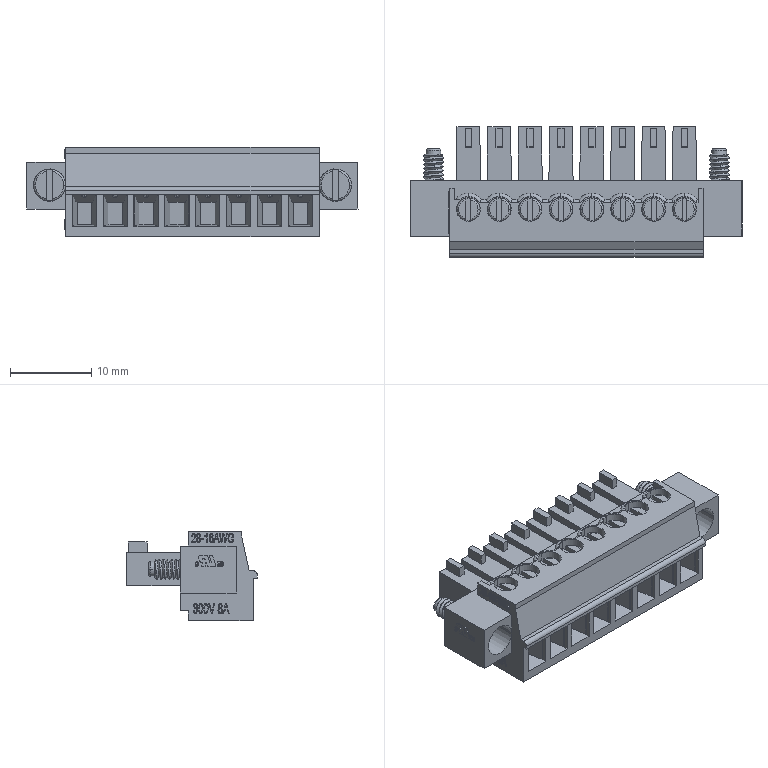Part | NX | features BREP 13 | 13 solids | 1134 faces | box 40.98 x 16.1 x 11 mm | volume 3428 mm3 | plane 533 | spline 275 | cylinder 186 | torus 104 | cone 36 | commonest cylinder face diameters 2.5 x26 1 x25 0.8 x24 2.8 x16 2.94 x16 4 x12